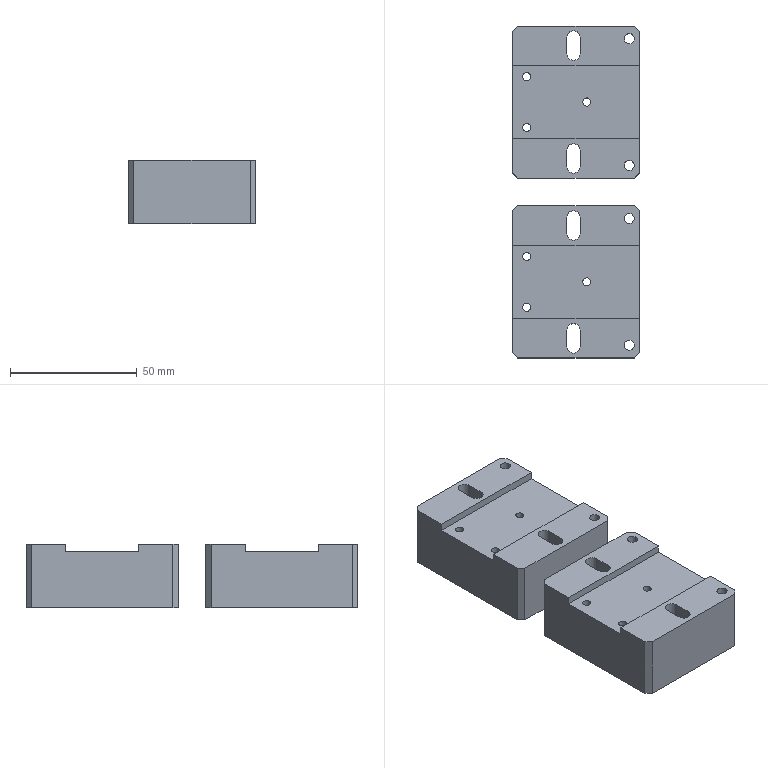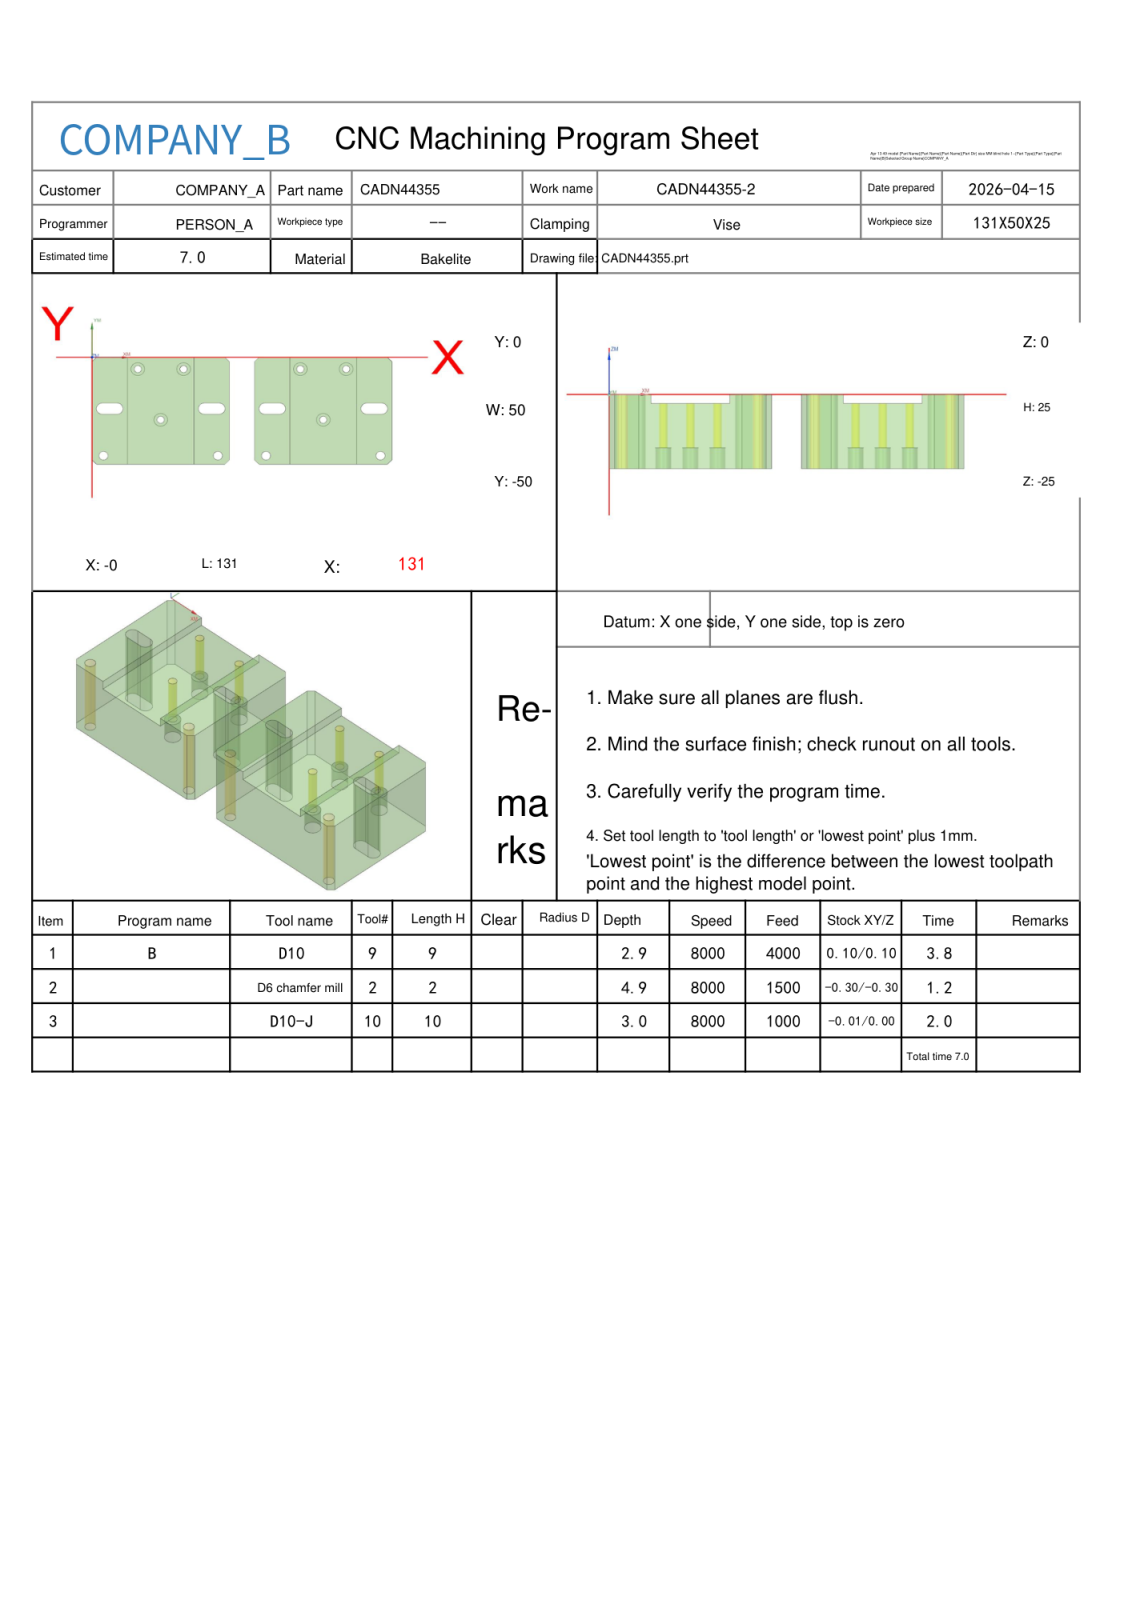NC program | NX | posted by the shop | part box 50 x 131 x 25 mm
Lines 1 to 802 of 4338:
%
O0001
(Machine time: 7.60 MIN)
(===Total Tool:3===)
(T9=D10     D=10.  R=0.   D-  H09 Z=-2.9  )
(T2=D6 chamfer mill   D=6.   R=0.   D-  H02 Z=-4.9  )
(T10=D10-J  D=10.  R=0.   D10 H10 Z=-3.   )
G80 G90 G17 G49 G40
G91 G28 Z0
M01
N1 T09 M06
(D10  D=10. R=0. H=09 ce=0.12 di=0.10)
G00 G90 G54 X28.991 Y13.6 M03 S8000
G43 H09 Z20.
M08
Z2.1
G01 X29.008 Y13.502 Z1.476 F4000.
X29.025 Y13.403 Z1.228
X29.042 Y13.305 Z1.046
X29.059 Y13.206 Z.9
X29.076 Y13.108 Z.777
X29.093 Y13.009 Z.672
X29.11 Y12.911 Z.58
X29.127 Y12.812 Z.5
X29.144 Y12.713 Z.43
X29.161 Y12.615 Z.368
X29.178 Y12.516 Z.314
X29.195 Y12.418 Z.267
X29.212 Y12.319 Z.227
X29.229 Y12.221 Z.192
X29.246 Y12.122 Z.164
X29.263 Y12.024 Z.14
X29.28 Y11.925 Z.123
X29.297 Y11.827 Z.11
X29.314 Y11.728 Z.103
X29.331 Y11.63 Z.1
X29.718 Y9.389
G03 X30.035 Y9.003 I.502 J.09
X33.822 Y8.43 I3.807 J12.364
X42.517 Y8.294 I8.695 J277.549
X44.371 Y8.3 I0.0 J277.686
G01 X131.38 Y8.277
G02 X137.354 Y4.1 I-.25 J-6.718
X138.606 Y-1.684 I-15.543 J-6.392
X138.806 Y-9.793 I-163.999 J-8.108
X138.798 Y-11.481 I-164.2 J0.0
G01 X138.779 Y-50.847
G02 X134.696 Y-56.806 I-6.689 J.204
X128.992 Y-58.092 I-6.383 J15.012
X120.82 Y-58.308 I-8.172 J154.264
X118.986 Y-58.297 I0.0 J154.48
G01 X-.307 Y-58.281
G02 X-6.242 Y-54.313 I.157 J6.658
X-7.592 Y-48.483 I14.663 J6.465
X-7.808 Y-40.348 I152.835 J8.135
X-7.798 Y-38.547 I153.052 J0.0
G01 X-7.781 Y.807
G02 X-3.823 Y6.738 I6.655 J-.155
X1.94 Y8.085 I6.436 J-14.524
X10.496 Y8.313 I8.556 J-160.452
X12.715 Y8.298 I0.0 J-160.68
X18.675 Y8.324 I5.959 J-683.816
X27.825 Y8.263 I0.0 J-683.842
G03 X40.459 Y7.607 I12.634 J121.294
X41.447 Y7.611 I0.0 J121.95
G01 X129.55 Y7.577
G02 X136.067 Y3.324 I-.411 J-7.749
X137.771 Y-2.843 I-14.525 J-7.331
X138.106 Y-11.396 I-108.782 J-8.552
X138.094 Y-13.054 I-109.117 J0.0
G01 X138.076 Y-49.049
G02 X133.893 Y-55.528 I-7.734 J.404
X127.593 Y-57.277 I-7.409 J14.463
X118.929 Y-57.608 I-8.664 J113.324
X117.172 Y-57.594 I0.0 J113.654
G01 X1.42 Y-57.574
G02 X-5.036 Y-53.369 I.449 J7.748
X-6.757 Y-47.273 I14.267 J7.319
X-7.11 Y-38.528 I108.167 J8.745
X-7.094 Y-36.713 I108.52 J0.0
G01 X-7.075 Y-.92
G02 X-2.934 Y5.499 I7.732 J-.442
X3.289 Y7.263 I7.389 J-14.206
X11.993 Y7.608 I8.704 J-109.478
X13.779 Y7.594 I0.0 J-109.823
X18.643 Y7.62 I4.863 J-445.607
X26.858 Y7.545 I0.0 J-445.633
G03 X43.992 Y6.885 I17.134 J222.072
X46.681 Y6.901 I0.0 J222.732
G01 X127.591 Y6.885
G02 X135.294 Y1.93 I-.199 J-8.775
X137.073 Y-4.867 I-16.681 J-7.995
X137.408 Y-14.121 I-127.437 J-9.254
X137.394 Y-15.989 I-127.772 J0.0
G01 X137.375 Y-47.268
G02 X132.433 Y-54.792 I-8.759 J.369
X125.844 Y-56.55 I-7.904 J16.392
X116.837 Y-56.904 I-9.007 J114.568
X115.214 Y-56.892 I0.0 J114.922
G01 X3.364 Y-56.881
G02 X-4.344 Y-51.826 I.263 J8.805
X-6.062 Y-45.221 I16.777 J7.891
X-6.41 Y-35.904 I124.802 J9.317
X-6.395 Y-33.96 I125.149 J0.0
G01 X-6.376 Y-2.75
G02 X-1.442 Y4.783 I8.771 J-.362
X5.153 Y6.549 I7.909 J-16.35
X14.545 Y6.909 I9.392 J-122.015
X16.483 Y6.894 I0.0 J-122.376
X19.763 Y6.922 I3.279 J-191.12
X27.89 Y6.749 I0.0 J-191.148
G03 X44.528 Y6.195 I16.638 J249.257
X46.472 Y6.202 I0.0 J249.812
G01 X125.98 Y6.18
G02 X134.573 Y.615 I-.106 J-9.581
X136.36 Y-6.472 I-18.365 J-8.399
X136.702 Y-15.797 I-127.035 J-9.325
X136.692 Y-17.383 I-127.376 J0.0
G01 X136.677 Y-45.513
G02 X131.02 Y-54.12 I-9.596 J.144
X123.989 Y-55.864 I-8.35 J18.623
X114.281 Y-56.208 I-9.709 J136.601
X112.308 Y-56.194 I0.0 J136.945
G01 X5.008 Y-56.177
G02 X-3.635 Y-50.483 I.137 J9.616
X-5.38 Y-43.309 I18.973 J8.413
X-5.701 Y-34.062 I133.064 J9.247
X-5.692 Y-32.537 I133.385 J0.0
G01 X-5.677 Y-4.477
G02 X-.024 Y4.115 I9.603 J-.162
X7.076 Y5.869 I8.395 J-18.743
X16.754 Y6.208 I9.678 J-137.942
X18.688 Y6.194 I0.0 J-138.281
X19.619 Y6.196 I.932 J-205.177
X33.13 Y5.751 I0.0 J-205.179
G03 X47.84 Y5.489 I14.711 J412.502
X51.091 Y5.502 I0.0 J412.764
G01 X124.371 Y5.481
X124.481
G02 X133.892 Y-.671 I0.0 J-10.274
X135.636 Y-7.774 I-19.734 J-8.61
X136.006 Y-17.723 I-133.543 J-9.949
X135.993 Y-19.595 I-133.913 J0.0
G01 X135.973 Y-44.014
G02 X129.816 Y-53.396 I-10.251 J.016
X122.705 Y-55.138 I-8.615 J19.79
X113.115 Y-55.5 I-9.59 J126.913
X111.585 Y-55.49 I0.0 J127.275
G01 X6.525 Y-55.474
X6.516
G02 X-2.927 Y-49.247 I0.0 J10.273
X-4.665 Y-41.915 I20.363 J8.699
X-5.01 Y-31.696 I151.073 J10.219
X-4.995 Y-29.533 I151.418 J0.0
G01 X-4.974 Y-6.023
Y-6.02
G02 X1.265 Y3.432 I10.279 J0.0
X8.657 Y5.171 I8.725 J-20.515
X19.005 Y5.512 I10.348 J-156.81
X21.809 Y5.487 I0.0 J-157.151
X34.788 Y4.993 I-10.339 J-442.411
G03 X48.798 Y4.798 I14.011 J502.746
X50.881 Y4.802 I0.0 J502.941
G01 X122.97 Y4.778
X123.087
G02 X129.785 Y2.576 I0.0 J-11.285
X133.941 Y-3.828 I-7.974 J-9.726
X135.128 Y-11.911 I-32.188 J-8.853
X135.314 Y-23.744 I-374.887 J-11.833
X135.298 Y-27.238 I-375.073 J0.0
X135.32 Y-32.951 I-730.277 J-5.713
X135.251 Y-42.978 I-730.299 J0.0
X128.729 Y-52.656 I-10.751 J.208
X121.344 Y-54.431 I-8.925 J20.885
X111.192 Y-54.803 I-10.152 J138.285
X109.383 Y-54.792 I0.0 J138.657
G01 X8.173 Y-54.779
X7.992 Y-54.78
G02 X1.676 Y-52.909 I0.0 J11.596
X-2.831 Y-46.511 I7.178 J9.842
X-4.109 Y-38.444 I30.132 J8.907
X-4.318 Y-26.37 I347.816 J12.074
X-4.298 Y-22.627 I348.025 J0.0
X-4.316 Y-17.155 I833.408 J5.472
X-4.255 Y-7.098 I833.426 J0.0
X2.351 Y2.691 I10.788 J-.157
X9.881 Y4.452 I8.982 J-21.435
X20.246 Y4.803 I10.365 J-152.514
X29.452 Y4.526 I0.0 J-152.866
G03 X48.789 Y4.087 I19.337 J425.155
X52.421 Y4.102 I0.0 J425.595
G01 X121.361 Y4.084
G02 X121.608 Y4.086 I.247 J-12.974
X127.696 Y2.569 I0.0 J-12.976
X132.862 Y-3.873 I-6.219 J-10.28
X134.345 Y-11.9 I-27.206 J-9.177
X134.607 Y-22.594 I-218.407 J-10.694
X134.595 Y-24.845 I-218.669 J0.0
X134.62 Y-31.239 I-841.387 J-6.394
X134.557 Y-41.495 I-841.412 J0.0
X132.207 Y-48.47 I-11.701 J.059
X125.63 Y-52.7 I-10.025 J8.36
X117.061 Y-53.933 I-9.262 J33.97
X105.122 Y-54.112 I-11.939 J398.216
X101.733 Y-54.097 I0.0 J398.395
G01 X9.693 Y-54.081
G02 X9.423 Y-54.083 I-.27 J13.123
X3.417 Y-52.629 I0.0 J13.125
X-1.873 Y-46.092 I6.097 J10.344
X-3.348 Y-38.058 I27.394 J9.179
X-3.612 Y-26.898 I235.667 J11.161
X-3.596 Y-24.203 I235.932 J0.0
X-3.622 Y-18.354 I675.776 J5.849
X-3.547 Y-8.324 I675.801 J0.0
X-.679 Y-.912 I11.402 J-.151
X5.93 Y2.861 I9.852 J-9.582
X14.172 Y3.943 I9.02 J-36.787
X20.494 Y4.044 I6.322 J-198.411
X32.011 Y3.709 I0.0 J-198.512
G03 X49.319 Y3.395 I17.308 J475.435
X52.071 Y3.403 I0.0 J475.75
G01 X120.1 Y3.381
G02 X120.332 Y3.383 I.231 J-14.118
X126.345 Y2.039 I0.0 J-14.12
X132.018 Y-4.584 I-5.761 J-10.675
X133.596 Y-12.52 I-26.22 J-9.34
X133.902 Y-22.992 I-179.256 J-10.473
X133.892 Y-24.833 I-179.561 J0.0
X133.916 Y-30.613 I-700.808 J-5.779
X133.848 Y-40.363 I-700.831 J0.0
X131.619 Y-47.33 I-12.343 J.109
X124.928 Y-51.869 I-10.361 J8.073
X116.654 Y-53.185 I-9.323 J31.945
X103.993 Y-53.418 I-12.66 J342.892
X100.137 Y-53.397 I0.0 J343.125
G01 X11.037 Y-53.38
G02 X10.745 Y-53.383 I-.292 J14.53
X4.908 Y-52.159 I0.0 J14.533
X-.864 Y-45.791 I5.363 J10.66
X-2.58 Y-37.671 I24.899 J9.504
X-2.904 Y-26.972 I176.35 J10.7
X-2.893 Y-24.938 I176.674 J0.0
X-2.917 Y-19.277 I669.743 J5.661
X-2.847 Y-9.619 I669.767 J0.0
X-.567 Y-2.602 I12.314 J-.122
X6.054 Y1.861 I10.318 J-8.163
X14.466 Y3.191 I9.39 J-32.128
X21.258 Y3.327 I6.792 J-169.694
X30.822 Y3.058 I0.0 J-169.83
G03 X49.688 Y2.696 I18.866 J491.676
X52.352 Y2.703 I0.0 J492.038
G01 X118.701 Y2.684
G02 X119.006 Y2.687 I.305 J-15.753
X124.921 Y1.534 I0.0 J-15.756
X131.096 Y-5.08 I-5.159 J-11.006
X132.851 Y-13.188 I-24.962 J-9.645
X133.206 Y-24.257 I-172.554 J-11.069
X133.192 Y-26.41 I-172.909 J0.0
X133.221 Y-31.121 I-388.488 J-4.711
X133.132 Y-39.419 I-388.517 J0.0
X130.819 Y-46.498 I-12.708 J.234
X123.931 Y-51.145 I-10.617 J8.308
X115.586 Y-52.474 I-9.483 J32.694
X103.39 Y-52.715 I-12.196 J308.696
X99.979 Y-52.696 I0.0 J308.937
G01 X12.209 Y-52.676
G02 X11.94 Y-52.679 I-.27 J15.48
X5.997 Y-51.493 I0.0 J15.483
X-.103 Y-44.899 I5.264 J10.988
X-1.834 Y-36.996 I24.74 J9.561
X-2.196 Y-26.516 I151.42 J10.48
X-2.189 Y-24.964 I151.782 J0.0
X-2.22 Y-19.549 I463.03 J5.415
X-2.134 Y-10.625 I463.062 J0.0
X.156 Y-3.536 I12.758 J-.206
X7.058 Y1.14 I10.632 J-8.261
X15.819 Y2.494 I9.634 J-33.33
X21.598 Y2.605 I5.779 J-149.809
X28.695 Y2.437 I0.0 J-149.92
G03 X50.48 Y1.993 I21.785 J534.705
X53.681 Y2.003 I0.0 J535.149
G01 X117.721 Y1.977
G02 X117.944 Y1.979 I.224 J-16.151
X124.072 Y.771 I0.0 J-16.152
X130.319 Y-5.897 I-5.302 J-11.226
X132.133 Y-14.14 I-25.167 J-9.86
X132.502 Y-25.226 I-166.047 J-11.086
X132.491 Y-27.221 I-166.417 J0.0
X132.517 Y-31.109 I-286.68 J-3.888
X132.425 Y-38.35 I-286.706 J0.0
X130.265 Y-45.351 I-13.312 J.274
X123.298 Y-50.314 I-10.905 J7.938
X114.833 Y-51.747 I-9.716 J31.677
X103.251 Y-52.008 I-11.583 J257.195
X100.627 Y-51.994 I0.0 J257.456
G01 X13.488 Y-51.977
G02 X13.167 Y-51.98 I-.32 J16.782
X7.183 Y-50.877 I0.0 J16.785
X.667 Y-44.06 I5.019 J11.321
X-1.142 Y-35.75 I25.417 J9.882
X-1.504 Y-24.559 I172.611 J11.191
X-1.491 Y-22.458 I172.974 J0.0
X-1.517 Y-18.721 I267.32 J3.737
X-1.423 Y-11.609 I267.346 J0.0
X.802 Y-4.554 I13.21 J-.287
X7.682 Y.307 I10.853 J-8.063
X16.566 Y1.763 I9.81 J-32.03
X22.392 Y1.871 I5.826 J-156.433
X30.245 Y1.674 I0.0 J-156.542
G03 X50.779 Y1.298 I20.533 J559.993
X53.401 Y1.304 I0.0 J560.37
G01 X116.461 Y1.279
G02 X116.725 Y1.281 I.265 J-17.642
X122.776 Y.212 I0.0 J-17.644
X129.519 Y-6.642 I-4.891 J-11.557
X131.39 Y-14.797 I-24.73 J-9.966
X131.795 Y-25.716 I-147.1 J-10.92
X131.787 Y-27.316 I-147.505 J0.0
X131.816 Y-30.779 I-205.435 J-3.463
X131.705 Y-37.535 I-205.465 J0.0
X129.296 Y-44.809 I-13.392 J.398
X122.157 Y-49.661 I-11.052 J8.584
X113.613 Y-51.052 I-9.827 J33.443
X102.137 Y-51.304 I-11.475 J260.365
X99.757 Y-51.293 I0.0 J260.617
G01 X14.507 Y-51.272
G02 X14.253 Y-51.274 I-.254 J17.512
X8.196 Y-50.193 I0.0 J17.514
X1.419 Y-43.208 I4.955 J11.587
X-.424 Y-34.829 I25.678 J10.039
X-.795 Y-23.964 I158.77 J10.865
X-.787 Y-22.378 I159.141 J0.0
X-.818 Y-19.042 I181.257 J3.336
X-.693 Y-12.3 I181.288 J0.0
X1.983 Y-4.828 I13.13 J-.487
X9.089 Y-.261 I10.942 J-9.212
X18.279 Y1.075 I9.797 J-35.115
X22.872 Y1.129 I4.594 J-194.707
X32.399 Y.896 I0.0 J-194.761
G03 X51.53 Y.6 I19.131 J617.569
X53.822 Y.604 I0.0 J617.865
G01 X115.341 Y.579
G02 X115.622 Y.581 I.281 J-18.556
X121.799 Y-.478 I0.0 J-18.558
X128.7 Y-7.319 I-4.802 J-11.744
X130.67 Y-15.662 I-24.529 J-10.196
X131.093 Y-26.67 I-143.146 J-11.008
X131.085 Y-28.181 I-143.568 J0.0
X131.116 Y-30.915 I-117.725 J-2.734
X130.955 Y-37.067 I-117.757 J0.0
X127.739 Y-44.966 I-13.016 J.696
X120.468 Y-49.176 I-10.969 J10.561
X111.26 Y-50.417 I-10.109 J40.22
X98.11 Y-50.612 I-13.15 J443.376
X94.253 Y-50.595 I0.0 J443.571
G01 X15.793 Y-50.575
G02 X15.448 Y-50.578 I-.344 J18.978
X9.325 Y-49.563 I0.0 J18.981
X2.287 Y-42.645 I4.668 J11.788
X.327 Y-34.299 I24.651 J10.192
X-.096 Y-23.072 I148.726 J11.226
X-.086 Y-21.36 I149.149 J0.0
X-.114 Y-18.864 I113.844 J2.496
X.036 Y-13.033 I113.872 J0.0
X3.057 Y-5.266 I13.152 J-.645
X10.406 Y-.862 I11.053 J-10.11
X19.611 Y.362 I9.631 J-37.194
X23.298 Y.392 I3.686 J-229.707
X33.785 Y.152 I0.0 J-229.737
G03 X52.625 Y-.101 I18.84 J701.361
X55.221 Y-.096 I0.0 J701.614
G01 X114.22 Y-.121
G02 X114.512 Y-.119 I.292 J-19.73
X120.694 Y-1.112 I0.0 J-19.732
X127.922 Y-8.073 I-4.577 J-11.987
X129.933 Y-16.339 I-24.292 J-10.285
X130.393 Y-27.633 I-138.428 J-11.294
X130.384 Y-29.206 I-138.888 J0.0
X130.413 Y-31.18 I-65.559 J-1.974
X130.17 Y-36.828 I-65.589 J0.0
X122.401 Y-47.432 I-12.776 J1.212
X114.067 Y-49.442 I-10.312 J24.484
X102.679 Y-49.894 I-11.388 J142.988
X100.989 Y-49.884 I0.0 J143.441
G01 X16.929 Y-49.875
G02 X16.563 Y-49.878 I-.367 J20.185
X10.381 Y-48.908 I0.0 J20.188
X2.989 Y-41.725 I4.539 J12.067
X1.052 Y-33.508 I25.002 J10.229
X.605 Y-22.084 I145.57 J11.424
X.615 Y-20.36 I146.017 J0.0
X.587 Y-18.55 I57.565 J1.81
X.86 Y-12.949 I57.594 J0.0
X8.573 Y-2.581 I12.732 J-1.418
X16.98 Y-.581 I10.123 J-23.883
X24.671 Y-.311 I7.691 J-109.422
X29.711 Y-.427 I0.0 J-109.692
G03 X53.526 Y-.806 I23.814 J747.153
X57.461 Y-.796 I0.0 J747.532
G01 X113.17 Y-.822
G02 X113.477 Y-.82 I.307 J-20.479
X119.785 Y-1.815 I0.0 J-20.482
X127.238 Y-9.014 I-4.604 J-12.223
X129.225 Y-17.286 I-24.928 J-10.364
X129.695 Y-28.872 I-142.779 J-11.586
X129.682 Y-30.783 I-143.248 J0.0
X129.699 Y-31.818 I-31.901 J-1.035
X129.181 Y-37.541 I-31.917 J0.0
X121.648 Y-46.662 I-12.629 J2.759
X113.46 Y-48.699 I-10.362 J24.181
X102.517 Y-49.18 I-10.943 J124.182
X101.505 Y-49.176 I0.0 J124.663
G01 X18.145
G02 X17.741 Y-49.18 I-.404 J22.153
X11.645 Y-48.325 I0.0 J22.157
X3.831 Y-41.132 I4.106 J12.301
X1.793 Y-32.878 I24.312 J10.383
X1.307 Y-21.269 I138.381 J11.609
X1.319 Y-19.452 I138.867 J0.0
X1.3 Y-18.324 I33.748 J1.128
X1.785 Y-12.62 I33.767 J0.0
X9.498 Y-3.274 I12.699 J-2.624
X17.983 Y-1.299 I10.147 J-24.373
X25.388 Y-1.047 I7.405 J-108.646
X29.945 Y-1.142 I0.0 J-108.898
G03 X53.166 Y-1.499 I23.22 J754.328
X55.712 Y-1.495 I0.0 J754.685
G01 X111.841 Y-1.516
G02 X112.234 Y-1.513 I.393 J-23.034
X118.413 Y-2.357 I0.0 J-23.037
X126.392 Y-9.587 I-4.04 J-12.476
X128.5 Y-18.042 I-24.396 J-10.572
X128.973 Y-28.635 I-118.47 J-10.593
X128.856 Y-33.915 I-118.943 J0.0
X126.411 Y-41.417 I-14.525 J.584
X119.028 Y-46.649 I-11.696 J8.68
X110.086 Y-48.204 I-10.439 J33.523
X97.779 Y-48.506 I-12.307 J251.03
X95.112 Y-48.492 I0.0 J251.332
G01 X19.032 Y-48.472
G02 X18.668 Y-48.475 I-.364 J22.235
X12.399 Y-47.573 I0.0 J22.238
X4.507 Y-40.19 I4.274 J12.477
X2.489 Y-31.852 I25.082 J10.483
X2.03 Y-21.252 I122.179 J10.6
X2.132 Y-16.258 I122.638 J0.0
X4.292 Y-9.027 I14.935 J-.523
X11.609 Y-3.488 I11.75 J-7.919
X20.679 Y-1.901 I9.969 J-30.27
X26.299 Y-1.796 I5.62 J-150.06
X31.876 Y-1.899 I0.0 J-150.165
G03 X54.589 Y-2.203 I22.713 J848.309
X58.301 Y-2.195 I0.0 J848.613
G01 X111.001 Y-2.22
G02 X111.325 Y-2.218 I.325 J-23.141
X117.639 Y-3.096 I0.0 J-23.143
X125.678 Y-10.432 I-4.152 J-12.624
X127.809 Y-19.097 I-25.013 J-10.745
X128.25 Y-28.31 I-95.997 J-9.213
X128.125 Y-33.221 I-96.438 J0.0
X125.414 Y-40.978 I-14.435 J.692
X118.008 Y-45.99 I-11.705 J9.318
X108.988 Y-47.51 I-10.514 J34.852
X96.716 Y-47.804 I-12.272 J256.568
X94.153 Y-47.791 I0.0 J256.861
G01 X20.033 Y-47.771
G02 X19.66 Y-47.774 I-.373 J22.936
X13.26 Y-46.863 I0.0 J22.939
X5.268 Y-39.447 I4.276 J12.621
X3.2 Y-30.981 I25.157 J10.632
X2.748 Y-21.767 I93.635 J9.214
X2.887 Y-16.649 I94.087 J0.0
X5.713 Y-8.859 I14.247 J-.761
X13.142 Y-3.978 I11.598 J-9.558
X22.461 Y-2.591 I9.835 J-34.084
X27.326 Y-2.545 I4.865 J-257.387
X36.97 Y-2.726 I0.0 J-257.433
G03 X54.37 Y-2.905 I17.399 J847.369
X58.441 Y-2.895 I0.0 J847.548
G01 X110.021 Y-2.921
G02 X110.371 Y-2.918 I.35 J-23.571
X116.865 Y-3.83 I0.0 J-23.574
X124.974 Y-11.286 I-4.257 J-12.768
X127.076 Y-19.743 I-25.043 J-10.714
X127.52 Y-27.982 I-76.248 J-8.239
X127.376 Y-32.674 I-76.692 J0.0
X124.217 Y-40.764 I-14.119 J.851
X116.703 Y-45.423 I-11.683 J10.453
X107.594 Y-46.836 I-10.549 J37.942
X95.476 Y-47.101 I-12.118 J277.555
X93.108 Y-47.091 I0.0 J277.82
G01 X21.018 Y-47.07
G02 X20.645 Y-47.073 I-.373 J23.73
X14.172 Y-46.173 I0.0 J23.733
X6.017 Y-38.688 I4.214 J12.776
X3.899 Y-30.021 I25.427 J10.803
X3.481 Y-21.999 I76.74 J8.022
X3.62 Y-17.368 I77.158 J0.0
X6.713 Y-9.321 I14.166 J-.827
X14.375 Y-4.582 I11.629 J-10.238
X23.714 Y-3.31 I9.706 J-36.335
X28.084 Y-3.278 I4.37 J-298.714
X38.29 Y-3.452 I0.0 J-298.746
G03 X54.266 Y-3.604 I15.976 J841.998
X58.231 Y-3.595 I0.0 J842.15
G01 X109.041 Y-3.621
G02 X109.367 Y-3.619 I.326 J-24.728
X115.824 Y-4.477 I0.0 J-24.73
X124.31 Y-12.216 I-4.09 J-13.005
X126.406 Y-20.963 I-26.123 J-10.886
X126.778 Y-27.734 I-61.474 J-6.771
X126.625 Y-32.076 I-61.845 J0.0
X122.885 Y-40.642 I-13.896 J.968
X115.229 Y-44.896 I-11.625 J11.907
X105.745 Y-46.184 I-10.68 J43.08
X92.463 Y-46.407 I-13.281 J394.348
X89.017 Y-46.392 I0.0 J394.572
G01 X22.318 Y-46.375
G02 X21.849 Y-46.379 I-.469 J26.562
X15.452 Y-45.598 I0.0 J26.566
X6.75 Y-37.909 I3.773 J13.039
X4.624 Y-29.312 I25.416 J10.848
X4.224 Y-22.249 I62.189 J7.064
X4.369 Y-17.99 I62.589 J0.0
X7.939 Y-9.549 I13.972 J-.934
X15.577 Y-5.202 I11.484 J-11.295
X25.071 Y-4.027 I9.65 J-39.015
X28.575 Y-4.011 I3.504 J-375.745
X39.819 Y-4.179 I0.0 J-375.761
G03 X54.898 Y-4.308 I15.079 J881.035
X59.771 Y-4.294 I0.0 J881.164
G01 X107.92 Y-4.318
G02 X108.323 Y-4.315 I.402 J-26.148
X114.85 Y-5.143 I0.0 J-26.151
X123.542 Y-12.912 I-3.926 J-13.14
X125.673 Y-21.578 I-25.753 J-10.929
X126.025 Y-27.451 I-48.842 J-5.872
X125.847 Y-31.639 I-49.194 J0.0
X117.53 Y-43.063 I-13.661 J1.206
X108.788 Y-45.187 I-10.951 J26.018
X97.391 Y-45.675 I-11.398 J132.914
X96.482 Y-45.672 I0.0 J133.402
G01 X22.993 Y-45.67
G02 X22.606 Y-45.672 I-.386 J25.582
X15.999 Y-44.805 I0.0 J25.585
X7.411 Y-36.979 I4.101 J13.126
X5.3 Y-28.166 I26.348 J10.97
X4.973 Y-22.566 I47.764 J5.599
X5.168 Y-18.244 I48.091 J0.0
X13.614 Y-6.904 I13.581 J-1.299
X22.388 Y-4.942 I10.308 J-25.508
X30.213 Y-4.705 I7.826 J-128.865
X34.702 Y-4.783 I0.0 J-129.103
G03 X54.939 Y-5.007 I20.238 J913.357
X59.841 Y-4.994 I0.0 J913.582
G01 X106.731 Y-5.014
G02 X107.223 Y-5.01 I.493 J-28.243
X113.809 Y-5.789 I0.0 J-28.247
X122.731 Y-13.504 I-3.686 J-13.279
X124.927 Y-22.078 I-25.042 J-10.983
X125.259 Y-27.159 I-38.706 J-5.081
X125.032 Y-31.365 I-39.038 J0.0
X116.982 Y-42.228 I-13.575 J1.645
X108.405 Y-44.429 I-10.99 J25.011
X96.542 Y-44.978 I-11.863 J127.966
X95.332 Y-44.972 I0.0 J128.515
G01 X24.293 Y-44.975
G02 X23.768 Y-44.979 I-.525 J28.175
X17.146 Y-44.19 I0.0 J28.18
X8.18 Y-36.296 I3.759 J13.309
X6.041 Y-27.626 I25.867 J10.98
X5.741 Y-22.815 I38.464 J4.812
X5.961 Y-18.687 I38.764 J0.0
X14.355 Y-7.659 I13.542 J-1.599
X23.263 Y-5.67 I10.407 J-25.666
X31.317 Y-5.432 I8.054 J-136.076
X35.927 Y-5.51 I0.0 J-136.315
G03 X54.993 Y-5.707 I19.066 J919.642
X59.981 Y-5.694 I0.0 J919.839
G01 X105.751 Y-5.714
G02 X106.246 Y-5.71 I.496 J-29.543
X112.834 Y-6.454 I0.0 J-29.547
X122.106 Y-14.492 I-3.571 J-13.486
X124.276 Y-23.506 I-26.193 J-11.074
X124.484 Y-26.939 I-28.186 J-3.433
X124.077 Y-31.734 I-28.394 J0.0
X116.376 Y-41.42 I-13.353 J2.712
X107.613 Y-43.717 I-11.161 J24.712
X95.568 Y-44.279 I-12.045 J128.963
X94.261 Y-44.272 I0.0 J129.524
G01 X25.181 Y-44.273
G02 X24.67 Y-44.278 I-.511 J28.751
X18.032 Y-43.501 I0.0 J28.756
X8.904 Y-35.524 I3.698 J13.442
X6.74 Y-26.652 I25.94 J11.027
X6.518 Y-23.07 I28.7 J3.582
X6.894 Y-18.422 I28.922 J0.0
X14.872 Y-8.513 I13.296 J-2.539
X23.275 Y-6.472 I10.315 J-24.152
X31.633 Y-6.153 I8.357 J-109.088
X34.816 Y-6.199 I0.0 J-109.408
G03 X54.748 Y-6.408 I19.931 J952.093
X59.981 Y-6.393 I0.0 J952.301
G01 X104.771 Y-6.413
G02 X105.306 Y-6.409 I.535 J-30.408
X111.995 Y-7.153 I0.0 J-30.413
X121.402 Y-15.302 I-3.561 J-13.615
X123.611 Y-25.227 I-26.433 J-11.092
X123.69 Y-26.989 I-19.521 J-1.763
X122.757 Y-32.967 I-19.6 J0.0
X115.281 Y-40.847 I-12.932 J4.781
X106.42 Y-43.052 I-11.182 J26.035
X94.777 Y-43.571 I-11.643 J130.388
X93.906 Y-43.568 I0.0 J130.906
G01 X26.086 Y-43.572
G02 X25.61 Y-43.576 I-.476 J29.869
X19.002 Y-42.836 I0.0 J29.873
X9.643 Y-34.789 I3.536 J13.579
X7.419 Y-25.218 I25.849 J11.049
X7.311 Y-23.112 I20.494 J2.107
X8.103 Y-17.456 I20.602 J0.0
X15.612 Y-9.266 I12.861 J-4.255
X24.15 Y-7.196 I10.412 J-24.302
X32.711 Y-6.876 I8.561 J-114.153
X35.971 Y-6.922 I0.0 J-114.474
G03 X54.829 Y-7.108 I18.857 J959.785
X60.121 Y-7.093 I0.0 J959.97
G01 X104.141 Y-7.118
G02 X104.596 Y-7.114 I.455 J-29.233
X111.426 Y-7.923 I0.0 J-29.236
X120.627 Y-15.95 I-3.775 J-13.614
X122.819 Y-26.401 I-23.828 J-10.452
X122.608 Y-29.707 I-26.019 J0.0
X115.021 Y-39.874 I-13.371 J2.064
X106.425 Y-42.248 I-11.215 J23.856
X94.514 Y-42.865 I-11.91 J114.693
X93.636 Y-42.862 I0.0 J115.309
G01 X29.106 Y-42.889
G02 X27.918 Y-42.903 I-1.188 J48.87
X21.357 Y-42.461 I0.0 J48.884
X10.268 Y-33.812 I2.083 J14.104
X8.183 Y-23.587 I24.03 J10.225
X8.381 Y-20.374 I26.115 J0.0
X16.21 Y-10.086 I13.26 J-1.968
X24.794 Y-7.942 I10.513 J-23.832
X33.508 Y-7.598 I8.713 J-110.053
X36.404 Y-7.636 I0.0 J-110.397
G03 X54.654 Y-7.807 I18.249 J974.856
X59.911 Y-7.792 I0.0 J975.027
G01 X103.091 Y-7.815
G02 X103.6 Y-7.811 I.509 J-30.856
X110.452 Y-8.582 I0.0 J-30.86
X119.934 Y-16.771 I-3.611 J-13.764
X121.954 Y-26.18 I-20.906 J-9.41
X121.76 Y-29.153 I-22.926 J0.0
X114.332 Y-39.106 I-13.244 J2.136
X105.819 Y-41.515 I-11.231 J23.443
X93.907 Y-42.16 I-11.912 J109.667
X93.172 Y-42.157 I0.0 J110.312
G01 X83.163 Y-42.19
X27.663 Y-42.167
G02 X27.256 Y-42.17 I-.406 J29.882
X20.512 Y-41.399 I0.0 J29.885
X11.057 Y-33.202 I3.648 J13.759
X9.048 Y-23.819 I20.905 J9.383
X9.236 Y-20.889 I22.914 J0.0
X16.76 Y-10.934 I13.07 J-2.058
X25.184 Y-8.715 I10.539 J-22.903
X34.112 Y-8.319 I8.928 J-100.599
X36.442 Y-8.346 I0.0 J-100.995
G03 X53.812 Y-8.5 I17.371 J983.273
X57.953 Y-8.491 I0.0 J983.426
G01 X102.461 Y-8.52
G02 X102.847 Y-8.517 I.386 J-30.489
X109.681 Y-9.293 I0.0 J-30.492
X119.275 Y-17.669 I-3.654 J-13.867
X121.058 Y-25.95 I-18.334 J-8.28
X120.871 Y-28.682 I-20.117 J0.0
X113.733 Y-38.287 I-13.026 J2.226
X105.313 Y-40.767 I-11.253 J22.675
X93.396 Y-41.452 I-11.917 J103.272
X92.81 Y-41.451 I0.0 J103.958
G01 X80.42 Y-41.49
X28.56 Y-41.467
G02 X28.129 Y-41.47 I-.431 J30.311
X21.27 Y-40.684 I0.0 J30.314
X11.737 Y-32.348 I3.696 J13.847
X9.945 Y-24.068 I18.237 J8.28
X10.141 Y-21.271 I20.029 J0.0
X17.487 Y-11.699 I12.861 J-2.266
X26.182 Y-9.422 I10.693 J-23.09
X35.421 Y-9.035 I9.239 J-110.226
X38.14 Y-9.069 I0.0 J-110.613
G03 X53.91 Y-9.199 I15.77 J956.378
X57.953 Y-9.19 I0.0 J956.508
G01 X90.324 Y-9.188
G02 X92.753 Y-8.98 I2.429 J-14.035
X95.183 Y-9.188 I0.0 J-14.244
X97.489 Y-9.169 I2.306 J-136.73
X105.186 Y-9.386 I0.0 J-136.749
X112.89 Y-11.698 I-.899 J-16.981
X119.137 Y-19.942 I-8.317 J-12.792
X120.134 Y-25.616 I-15.645 J-5.673
X119.733 Y-29.247 I-16.642 J0.0
X112.889 Y-37.593 I-12.665 J3.406
X104.4 Y-40.075 I-11.281 J22.834
X92.539 Y-40.75 I-11.861 J103.81
X92.036 Y-40.749 I0.0 J104.485
G01 X79.226 Y-40.79
X29.536 Y-40.768
G02 X29.089 Y-40.771 I-.447 J31.831
X22.24 Y-40.026 I0.0 J31.834
X12.383 Y-31.409 I3.508 J13.96
X10.877 Y-24.323 I15.915 J7.086
X11.099 Y-21.549 I17.422 J0.0
X17.922 Y-12.62 I12.525 J-2.5
X26.368 Y-10.219 I10.704 J-21.596
X35.81 Y-9.756 I9.443 J-95.908
X37.832 Y-9.777 I0.0 J-96.372
G01 X57.045 Y-9.889
X87.78
G02 X90.324 Y-9.188 I5.685 J-15.672
G01 X90.379 Y-9.159 Z.127
X90.449 Y-9.086 Z.172
X90.475 Y-9.067 Z.186
X90.505 Y-9.056 Z.2
X91.144 Y-8.968
X91.786 Y-8.909
X92.431 Y-8.88
X93.076
X93.72 Y-8.909
X94.363 Y-8.968
X95.002 Y-9.056
X95.032 Y-9.067 Z.186
X95.058 Y-9.086 Z.172
X95.128 Y-9.159 Z.127
X95.183 Y-9.188 Z.1
G02 X97.736 Y-9.893 I-3.13 J-16.328
X99.048 Y-9.878 I1.312 J-60.853
X106.015 Y-10.278 I0.0 J-60.867
X115.16 Y-14.964 I-1.706 J-14.6
X119.148 Y-25.529 I-12. J-10.565
X119.008 Y-27.645 I-15.988 J0.0
X112.662 Y-36.552 I-12.434 J2.145
X104.527 Y-39.228 I-11.247 J20.483
X92.706 Y-40.029 I-11.822 J86.845
G01 X92.524
G02 X82.069 Y-40.1 I-10.454 J773.914
X78.104 Y-40.09 I0.0 J773.984
G01 X30.724 Y-40.072
G02 X30.159 Y-40.077 I-.565 J34.447
X23.281 Y-39.383 I0.0 J34.451
X12.92 Y-30.145 I3.246 J14.071
X11.845 Y-24.644 I13.543 J5.501
X12.338 Y-20.877 I14.618 J0.0
X19.01 Y-13.21 I12.137 J-3.823
X27.211 Y-10.942 I10.533 J-22.125
X36.822 Y-10.472 I9.611 J-97.986
X38.815 Y-10.492 I0.0 J-98.456
G01 X60.611 Y-10.591
X86.228 Y-10.59
X87.78 Y-9.889
X87.828 Y-9.85 Z.127
X87.883 Y-9.765 Z.172
X87.905 Y-9.741 Z.186
X87.933 Y-9.725 Z.2
X88.6 Y-9.502
X89.277 Y-9.311
X89.963 Y-9.155
X90.656 Y-9.033
X91.354 Y-8.946
X92.055 Y-8.893
X92.758 Y-8.876
X93.461 Y-8.894
X94.163 Y-8.947
X94.861 Y-9.034
X95.553 Y-9.157
X96.239 Y-9.314
X96.916 Y-9.504
X97.583 Y-9.729
X97.611 Y-9.745 Z.186
X97.632 Y-9.768 Z.172
X97.688 Y-9.854 Z.127
X97.736 Y-9.893 Z.1
X99.381 Y-10.612
G02 X99.94 Y-10.608 I.56 J-35.296
X106.894 Y-11.3 I0.0 J-35.3
X117.868 Y-22.605 I-3.162 J-14.047
X118.15 Y-25.202 I-11.795 J-2.596
X112.257 Y-35.576 I-12.078 J0.0
X104.043 Y-38.467 I-11.352 J19.138
X92.395 Y-39.315 I-11.696 J80.196
X81.108 Y-39.398 I-11.287 J768.755
X77.415 Y-39.389 I0.0 J768.838
G01 X31.295 Y-39.367
G02 X30.817 Y-39.371 I-.478 J33.009
X23.858 Y-38.629 I0.0 J33.013
X13.113 Y-27.276 I3.397 J13.977
X12.855 Y-24.814 I11.615 J2.463
X18.765 Y-14.547 I11.873 J0.0